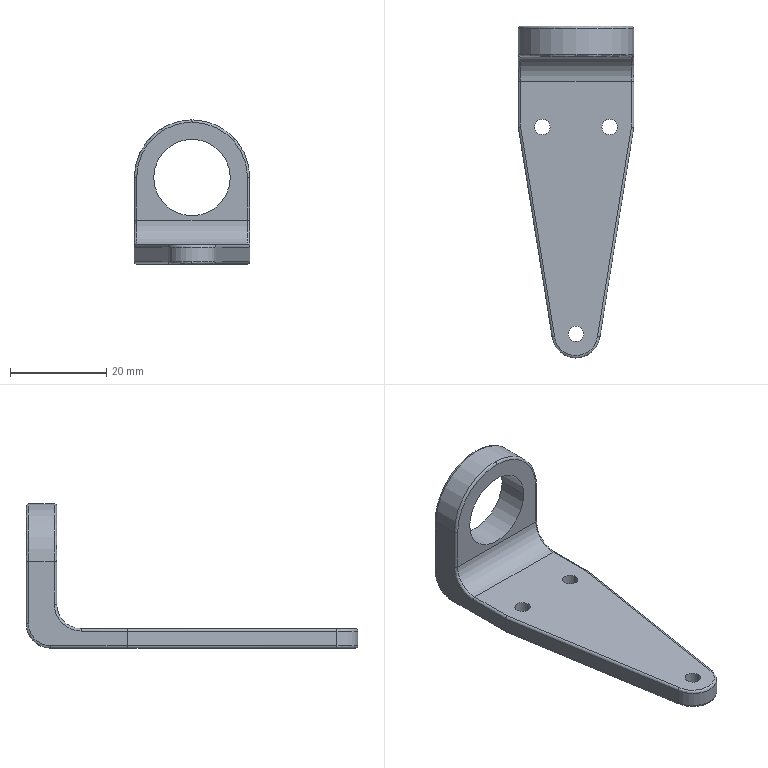Part | SolidWorks | features BaseBody 1 | 1 solid | 42 faces | box 24 x 68.952 x 30 mm | volume 7366 mm3 | cylinder 24 | spline 10 | plane 8 | commonest cylinder face diameters 1 x12 3.2 x6 10.16 x2 15.9 x2 10 x1 24 x1